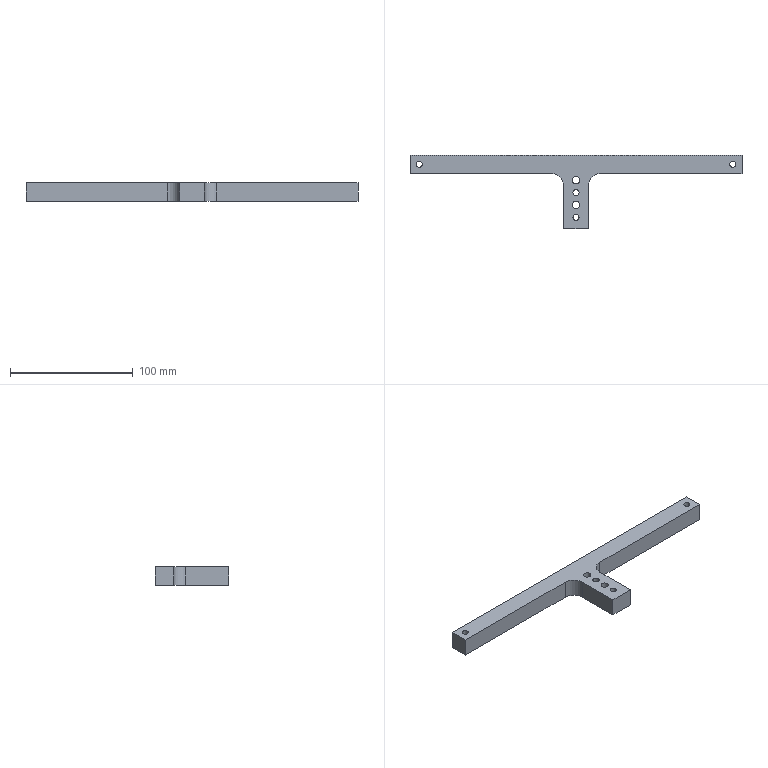Part | NX | features BREP 1 | 1 solid | 18 faces | box 270 x 60 x 15 mm | volume 72867 mm3 | plane 10 | cylinder 8 | commonest cylinder face diameters 5 x4 6 x2 20 x2
STEP:
#1=CARTESIAN_POINT('',(-10.,35.,7.5));
#2=VERTEX_POINT('',#1);
#3=CARTESIAN_POINT('',(-10.,0.,7.5));
#4=VERTEX_POINT('',#3);
#5=CARTESIAN_POINT('',(-10.,45.,7.5));
#6=DIRECTION('',(0.,-1.,0.));
#7=VECTOR('',#6,1000.);
#8=LINE('',#5,#7);
#9=EDGE_CURVE('',#2,#4,#8,.T.);
#10=ORIENTED_EDGE('',*,*,#9,.F.);
#11=CARTESIAN_POINT('',(-10.,35.,-7.5));
#12=VERTEX_POINT('',#11);
#13=CARTESIAN_POINT('',(-10.,35.,-7.5));
#14=DIRECTION('',(0.,0.,-1.));
#15=VECTOR('',#14,1000.);
#16=LINE('',#13,#15);
#17=EDGE_CURVE('',#2,#12,#16,.T.);
#18=ORIENTED_EDGE('',*,*,#17,.T.);
#19=CARTESIAN_POINT('',(-10.,0.,-7.5));
#20=VERTEX_POINT('',#19);
#21=CARTESIAN_POINT('',(-10.,45.,-7.5));
#22=DIRECTION('',(0.,-1.,0.));
#23=VECTOR('',#22,1000.);
#24=LINE('',#21,#23);
#25=EDGE_CURVE('',#12,#20,#24,.T.);
#26=ORIENTED_EDGE('',*,*,#25,.T.);
#27=CARTESIAN_POINT('',(-10.,0.,7.5));
#28=DIRECTION('',(0.,0.,-1.));
#29=VECTOR('',#28,1000.);
#30=LINE('',#27,#29);
#31=EDGE_CURVE('',#4,#20,#30,.T.);
#32=ORIENTED_EDGE('',*,*,#31,.F.);
#33=EDGE_LOOP('',(#10,#18,#26,#32));
#34=FACE_BOUND('',#33,.T.);
#35=CARTESIAN_POINT('',(-10.,45.,7.5));
#36=DIRECTION('',(1.,0.,0.));
#37=DIRECTION('',(0.,-1.,0.));
#38=AXIS2_PLACEMENT_3D('',#35,#36,#37);
#39=PLANE('',#38);
#40=ADVANCED_FACE('',(#34),#39,.F.);
#41=CARTESIAN_POINT('',(10.,0.,-7.5));
#42=VERTEX_POINT('',#41);
#43=CARTESIAN_POINT('',(-10.,0.,-7.5));
#44=DIRECTION('',(1.,0.,0.));
#45=VECTOR('',#44,1000.);
#46=LINE('',#43,#45);
#47=EDGE_CURVE('',#20,#42,#46,.T.);
#48=ORIENTED_EDGE('',*,*,#47,.T.);
#49=CARTESIAN_POINT('',(10.,0.,7.5));
#50=VERTEX_POINT('',#49);
#51=CARTESIAN_POINT('',(10.,0.,7.5));
#52=DIRECTION('',(0.,0.,-1.));
#53=VECTOR('',#52,1000.);
#54=LINE('',#51,#53);
#55=EDGE_CURVE('',#50,#42,#54,.T.);
#56=ORIENTED_EDGE('',*,*,#55,.F.);
#57=CARTESIAN_POINT('',(-10.,0.,7.5));
#58=DIRECTION('',(1.,0.,0.));
#59=VECTOR('',#58,1000.);
#60=LINE('',#57,#59);
#61=EDGE_CURVE('',#4,#50,#60,.T.);
#62=ORIENTED_EDGE('',*,*,#61,.F.);
#63=ORIENTED_EDGE('',*,*,#31,.T.);
#64=EDGE_LOOP('',(#48,#56,#62,#63));
#65=FACE_BOUND('',#64,.T.);
#66=CARTESIAN_POINT('',(-10.,0.,7.5));
#67=DIRECTION('',(0.,1.,0.));
#68=DIRECTION('',(0.,0.,-1.));
#69=AXIS2_PLACEMENT_3D('',#66,#67,#68);
#70=PLANE('',#69);
#71=ADVANCED_FACE('',(#65),#70,.F.);
#72=CARTESIAN_POINT('',(10.,35.,-7.5));
#73=VERTEX_POINT('',#72);
#74=CARTESIAN_POINT('',(10.,0.,-7.5));
#75=DIRECTION('',(0.,1.,0.));
#76=VECTOR('',#75,1000.);
#77=LINE('',#74,#76);
#78=EDGE_CURVE('',#42,#73,#77,.T.);
#79=ORIENTED_EDGE('',*,*,#78,.T.);
#80=CARTESIAN_POINT('',(10.,35.,7.5));
#81=VERTEX_POINT('',#80);
#82=CARTESIAN_POINT('',(10.,35.,7.5));
#83=DIRECTION('',(0.,0.,1.));
#84=VECTOR('',#83,1000.);
#85=LINE('',#82,#84);
#86=EDGE_CURVE('',#73,#81,#85,.T.);
#87=ORIENTED_EDGE('',*,*,#86,.T.);
#88=CARTESIAN_POINT('',(10.,0.,7.5));
#89=DIRECTION('',(0.,1.,0.));
#90=VECTOR('',#89,1000.);
#91=LINE('',#88,#90);
#92=EDGE_CURVE('',#50,#81,#91,.T.);
#93=ORIENTED_EDGE('',*,*,#92,.F.);
#94=ORIENTED_EDGE('',*,*,#55,.T.);
#95=EDGE_LOOP('',(#79,#87,#93,#94));
#96=FACE_BOUND('',#95,.T.);
#97=CARTESIAN_POINT('',(10.,0.,7.5));
#98=DIRECTION('',(-1.,0.,0.));
#99=DIRECTION('',(0.,1.,0.));
#100=AXIS2_PLACEMENT_3D('',#97,#98,#99);
#101=PLANE('',#100);
#102=ADVANCED_FACE('',(#96),#101,.F.);
#103=CARTESIAN_POINT('',(20.,45.,7.5));
#104=VERTEX_POINT('',#103);
#105=CARTESIAN_POINT('',(135.,45.,7.5));
#106=VERTEX_POINT('',#105);
#107=CARTESIAN_POINT('',(10.,45.,7.5));
#108=DIRECTION('',(1.,0.,0.));
#109=VECTOR('',#108,1000.);
#110=LINE('',#107,#109);
#111=EDGE_CURVE('',#104,#106,#110,.T.);
#112=ORIENTED_EDGE('',*,*,#111,.F.);
#113=CARTESIAN_POINT('',(20.,45.,-7.5));
#114=VERTEX_POINT('',#113);
#115=CARTESIAN_POINT('',(20.,45.,-7.5));
#116=DIRECTION('',(0.,0.,-1.));
#117=VECTOR('',#116,1000.);
#118=LINE('',#115,#117);
#119=EDGE_CURVE('',#104,#114,#118,.T.);
#120=ORIENTED_EDGE('',*,*,#119,.T.);
#121=CARTESIAN_POINT('',(135.,45.,-7.5));
#122=VERTEX_POINT('',#121);
#123=CARTESIAN_POINT('',(10.,45.,-7.5));
#124=DIRECTION('',(1.,0.,0.));
#125=VECTOR('',#124,1000.);
#126=LINE('',#123,#125);
#127=EDGE_CURVE('',#114,#122,#126,.T.);
#128=ORIENTED_EDGE('',*,*,#127,.T.);
#129=CARTESIAN_POINT('',(135.,45.,7.5));
#130=DIRECTION('',(0.,0.,-1.));
#131=VECTOR('',#130,1000.);
#132=LINE('',#129,#131);
#133=EDGE_CURVE('',#106,#122,#132,.T.);
#134=ORIENTED_EDGE('',*,*,#133,.F.);
#135=EDGE_LOOP('',(#112,#120,#128,#134));
#136=FACE_BOUND('',#135,.T.);
#137=CARTESIAN_POINT('',(10.,45.,7.5));
#138=DIRECTION('',(0.,1.,0.));
#139=DIRECTION('',(0.,0.,-1.));
#140=AXIS2_PLACEMENT_3D('',#137,#138,#139);
#141=PLANE('',#140);
#142=ADVANCED_FACE('',(#136),#141,.F.);
#143=CARTESIAN_POINT('',(135.,60.,-7.5));
#144=VERTEX_POINT('',#143);
#145=CARTESIAN_POINT('',(135.,45.,-7.5));
#146=DIRECTION('',(0.,1.,0.));
#147=VECTOR('',#146,1000.);
#148=LINE('',#145,#147);
#149=EDGE_CURVE('',#122,#144,#148,.T.);
#150=ORIENTED_EDGE('',*,*,#149,.T.);
#151=CARTESIAN_POINT('',(135.,60.,7.5));
#152=VERTEX_POINT('',#151);
#153=CARTESIAN_POINT('',(135.,60.,7.5));
#154=DIRECTION('',(0.,0.,-1.));
#155=VECTOR('',#154,1000.);
#156=LINE('',#153,#155);
#157=EDGE_CURVE('',#152,#144,#156,.T.);
#158=ORIENTED_EDGE('',*,*,#157,.F.);
#159=CARTESIAN_POINT('',(135.,45.,7.5));
#160=DIRECTION('',(0.,1.,0.));
#161=VECTOR('',#160,1000.);
#162=LINE('',#159,#161);
#163=EDGE_CURVE('',#106,#152,#162,.T.);
#164=ORIENTED_EDGE('',*,*,#163,.F.);
#165=ORIENTED_EDGE('',*,*,#133,.T.);
#166=EDGE_LOOP('',(#150,#158,#164,#165));
#167=FACE_BOUND('',#166,.T.);
#168=CARTESIAN_POINT('',(135.,45.,7.5));
#169=DIRECTION('',(-1.,0.,0.));
#170=DIRECTION('',(0.,0.,-1.));
#171=AXIS2_PLACEMENT_3D('',#168,#169,#170);
#172=PLANE('',#171);
#173=ADVANCED_FACE('',(#167),#172,.F.);
#174=CARTESIAN_POINT('',(-135.,60.,-7.5));
#175=VERTEX_POINT('',#174);
#176=CARTESIAN_POINT('',(135.,60.,-7.5));
#177=DIRECTION('',(-1.,0.,0.));
#178=VECTOR('',#177,1000.);
#179=LINE('',#176,#178);
#180=EDGE_CURVE('',#144,#175,#179,.T.);
#181=ORIENTED_EDGE('',*,*,#180,.T.);
#182=CARTESIAN_POINT('',(-135.,60.,7.5));
#183=VERTEX_POINT('',#182);
#184=CARTESIAN_POINT('',(-135.,60.,7.5));
#185=DIRECTION('',(0.,0.,-1.));
#186=VECTOR('',#185,1000.);
#187=LINE('',#184,#186);
#188=EDGE_CURVE('',#183,#175,#187,.T.);
#189=ORIENTED_EDGE('',*,*,#188,.F.);
#190=CARTESIAN_POINT('',(135.,60.,7.5));
#191=DIRECTION('',(-1.,0.,0.));
#192=VECTOR('',#191,1000.);
#193=LINE('',#190,#192);
#194=EDGE_CURVE('',#152,#183,#193,.T.);
#195=ORIENTED_EDGE('',*,*,#194,.F.);
#196=ORIENTED_EDGE('',*,*,#157,.T.);
#197=EDGE_LOOP('',(#181,#189,#195,#196));
#198=FACE_BOUND('',#197,.T.);
#199=CARTESIAN_POINT('',(135.,60.,7.5));
#200=DIRECTION('',(0.,-1.,0.));
#201=DIRECTION('',(0.,0.,1.));
#202=AXIS2_PLACEMENT_3D('',#199,#200,#201);
#203=PLANE('',#202);
#204=ADVANCED_FACE('',(#198),#203,.F.);
#205=CARTESIAN_POINT('',(-135.,45.,-7.5));
#206=VERTEX_POINT('',#205);
#207=CARTESIAN_POINT('',(-135.,60.,-7.5));
#208=DIRECTION('',(0.,-1.,0.));
#209=VECTOR('',#208,1000.);
#210=LINE('',#207,#209);
#211=EDGE_CURVE('',#175,#206,#210,.T.);
#212=ORIENTED_EDGE('',*,*,#211,.T.);
#213=CARTESIAN_POINT('',(-135.,45.,7.5));
#214=VERTEX_POINT('',#213);
#215=CARTESIAN_POINT('',(-135.,45.,7.5));
#216=DIRECTION('',(0.,0.,-1.));
#217=VECTOR('',#216,1000.);
#218=LINE('',#215,#217);
#219=EDGE_CURVE('',#214,#206,#218,.T.);
#220=ORIENTED_EDGE('',*,*,#219,.F.);
#221=CARTESIAN_POINT('',(-135.,60.,7.5));
#222=DIRECTION('',(0.,-1.,0.));
#223=VECTOR('',#222,1000.);
#224=LINE('',#221,#223);
#225=EDGE_CURVE('',#183,#214,#224,.T.);
#226=ORIENTED_EDGE('',*,*,#225,.F.);
#227=ORIENTED_EDGE('',*,*,#188,.T.);
#228=EDGE_LOOP('',(#212,#220,#226,#227));
#229=FACE_BOUND('',#228,.T.);
#230=CARTESIAN_POINT('',(-135.,60.,7.5));
#231=DIRECTION('',(1.,0.,0.));
#232=DIRECTION('',(0.,0.,1.));
#233=AXIS2_PLACEMENT_3D('',#230,#231,#232);
#234=PLANE('',#233);
#235=ADVANCED_FACE('',(#229),#234,.F.);
#236=CARTESIAN_POINT('',(-20.,45.,-7.5));
#237=VERTEX_POINT('',#236);
#238=CARTESIAN_POINT('',(-135.,45.,-7.5));
#239=DIRECTION('',(1.,0.,0.));
#240=VECTOR('',#239,1000.);
#241=LINE('',#238,#240);
#242=EDGE_CURVE('',#206,#237,#241,.T.);
#243=ORIENTED_EDGE('',*,*,#242,.T.);
#244=CARTESIAN_POINT('',(-20.,45.,7.5));
#245=VERTEX_POINT('',#244);
#246=CARTESIAN_POINT('',(-20.,45.,7.5));
#247=DIRECTION('',(0.,0.,1.));
#248=VECTOR('',#247,1000.);
#249=LINE('',#246,#248);
#250=EDGE_CURVE('',#237,#245,#249,.T.);
#251=ORIENTED_EDGE('',*,*,#250,.T.);
#252=CARTESIAN_POINT('',(-135.,45.,7.5));
#253=DIRECTION('',(1.,0.,0.));
#254=VECTOR('',#253,1000.);
#255=LINE('',#252,#254);
#256=EDGE_CURVE('',#214,#245,#255,.T.);
#257=ORIENTED_EDGE('',*,*,#256,.F.);
#258=ORIENTED_EDGE('',*,*,#219,.T.);
#259=EDGE_LOOP('',(#243,#251,#257,#258));
#260=FACE_BOUND('',#259,.T.);
#261=CARTESIAN_POINT('',(-135.,45.,7.5));
#262=DIRECTION('',(0.,1.,0.));
#263=DIRECTION('',(0.,0.,-1.));
#264=AXIS2_PLACEMENT_3D('',#261,#262,#263);
#265=PLANE('',#264);
#266=ADVANCED_FACE('',(#260),#265,.F.);
#267=CARTESIAN_POINT('',(-125.,52.5,7.5));
#268=VERTEX_POINT('',#267);
#269=CARTESIAN_POINT('',(-127.5,52.5,7.5));
#270=DIRECTION('',(0.,0.,1.));
#271=DIRECTION('',(1.,0.,0.));
#272=AXIS2_PLACEMENT_3D('',#269,#270,#271);
#273=CIRCLE('',#272,2.5);
#274=EDGE_CURVE('',#268,#268,#273,.T.);
#275=ORIENTED_EDGE('',*,*,#274,.F.);
#276=EDGE_LOOP('',(#275));
#277=FACE_BOUND('',#276,.T.);
#278=CARTESIAN_POINT('',(130.,52.5,7.5));
#279=VERTEX_POINT('',#278);
#280=CARTESIAN_POINT('',(127.5,52.5,7.5));
#281=DIRECTION('',(0.,0.,1.));
#282=DIRECTION('',(1.,0.,0.));
#283=AXIS2_PLACEMENT_3D('',#280,#281,#282);
#284=CIRCLE('',#283,2.5);
#285=EDGE_CURVE('',#279,#279,#284,.T.);
#286=ORIENTED_EDGE('',*,*,#285,.F.);
#287=EDGE_LOOP('',(#286));
#288=FACE_BOUND('',#287,.T.);
#289=CARTESIAN_POINT('',(-2.5,9.5,7.5));
#290=VERTEX_POINT('',#289);
#291=CARTESIAN_POINT('',(0.,9.5,7.5));
#292=DIRECTION('',(0.,0.,-1.));
#293=DIRECTION('',(-1.,0.,0.));
#294=AXIS2_PLACEMENT_3D('',#291,#292,#293);
#295=CIRCLE('',#294,2.5);
#296=EDGE_CURVE('',#290,#290,#295,.T.);
#297=ORIENTED_EDGE('',*,*,#296,.T.);
#298=EDGE_LOOP('',(#297));
#299=FACE_BOUND('',#298,.T.);
#300=CARTESIAN_POINT('',(-2.5,29.5,7.5));
#301=VERTEX_POINT('',#300);
#302=CARTESIAN_POINT('',(0.,29.5,7.5));
#303=DIRECTION('',(0.,0.,-1.));
#304=DIRECTION('',(-1.,0.,0.));
#305=AXIS2_PLACEMENT_3D('',#302,#303,#304);
#306=CIRCLE('',#305,2.5);
#307=EDGE_CURVE('',#301,#301,#306,.T.);
#308=ORIENTED_EDGE('',*,*,#307,.T.);
#309=EDGE_LOOP('',(#308));
#310=FACE_BOUND('',#309,.T.);
#311=CARTESIAN_POINT('',(3.,19.5,7.5));
#312=VERTEX_POINT('',#311);
#313=CARTESIAN_POINT('',(0.,19.5,7.5));
#314=DIRECTION('',(0.,0.,1.));
#315=DIRECTION('',(1.,0.,0.));
#316=AXIS2_PLACEMENT_3D('',#313,#314,#315);
#317=CIRCLE('',#316,3.);
#318=EDGE_CURVE('',#312,#312,#317,.T.);
#319=ORIENTED_EDGE('',*,*,#318,.F.);
#320=EDGE_LOOP('',(#319));
#321=FACE_BOUND('',#320,.T.);
#322=CARTESIAN_POINT('',(3.,39.5,7.5));
#323=VERTEX_POINT('',#322);
#324=CARTESIAN_POINT('',(0.,39.5,7.5));
#325=DIRECTION('',(0.,0.,1.));
#326=DIRECTION('',(1.,0.,0.));
#327=AXIS2_PLACEMENT_3D('',#324,#325,#326);
#328=CIRCLE('',#327,3.);
#329=EDGE_CURVE('',#323,#323,#328,.T.);
#330=ORIENTED_EDGE('',*,*,#329,.F.);
#331=EDGE_LOOP('',(#330));
#332=FACE_BOUND('',#331,.T.);
#333=ORIENTED_EDGE('',*,*,#256,.T.);
#334=CARTESIAN_POINT('',(-20.,35.,7.5));
#335=DIRECTION('',(0.,0.,-1.));
#336=DIRECTION('',(1.,0.,0.));
#337=AXIS2_PLACEMENT_3D('',#334,#335,#336);
#338=CIRCLE('',#337,10.);
#339=EDGE_CURVE('',#245,#2,#338,.T.);
#340=ORIENTED_EDGE('',*,*,#339,.T.);
#341=ORIENTED_EDGE('',*,*,#9,.T.);
#342=ORIENTED_EDGE('',*,*,#61,.T.);
#343=ORIENTED_EDGE('',*,*,#92,.T.);
#344=CARTESIAN_POINT('',(20.,35.,7.5));
#345=DIRECTION('',(0.,0.,-1.));
#346=DIRECTION('',(1.,0.,0.));
#347=AXIS2_PLACEMENT_3D('',#344,#345,#346);
#348=CIRCLE('',#347,10.);
#349=EDGE_CURVE('',#81,#104,#348,.T.);
#350=ORIENTED_EDGE('',*,*,#349,.T.);
#351=ORIENTED_EDGE('',*,*,#111,.T.);
#352=ORIENTED_EDGE('',*,*,#163,.T.);
#353=ORIENTED_EDGE('',*,*,#194,.T.);
#354=ORIENTED_EDGE('',*,*,#225,.T.);
#355=EDGE_LOOP('',(#333,#340,#341,#342,#343,#350,#351,#352,#353,#354));
#356=FACE_BOUND('',#355,.T.);
#357=CARTESIAN_POINT('',(0.,0.,7.5));
#358=DIRECTION('',(0.,0.,1.));
#359=DIRECTION('',(-1.,0.,0.));
#360=AXIS2_PLACEMENT_3D('',#357,#358,#359);
#361=PLANE('',#360);
#362=ADVANCED_FACE('',(#277,#288,#299,#310,#321,#332,#356),#361,.T.);
#363=CARTESIAN_POINT('',(-125.,52.5,-7.5));
#364=VERTEX_POINT('',#363);
#365=CARTESIAN_POINT('',(-127.5,52.5,-7.5));
#366=DIRECTION('',(0.,0.,1.));
#367=DIRECTION('',(1.,0.,0.));
#368=AXIS2_PLACEMENT_3D('',#365,#366,#367);
#369=CIRCLE('',#368,2.5);
#370=EDGE_CURVE('',#364,#364,#369,.T.);
#371=ORIENTED_EDGE('',*,*,#370,.T.);
#372=EDGE_LOOP('',(#371));
#373=FACE_BOUND('',#372,.T.);
#374=CARTESIAN_POINT('',(130.,52.5,-7.5));
#375=VERTEX_POINT('',#374);
#376=CARTESIAN_POINT('',(127.5,52.5,-7.5));
#377=DIRECTION('',(0.,0.,1.));
#378=DIRECTION('',(1.,0.,0.));
#379=AXIS2_PLACEMENT_3D('',#376,#377,#378);
#380=CIRCLE('',#379,2.5);
#381=EDGE_CURVE('',#375,#375,#380,.T.);
#382=ORIENTED_EDGE('',*,*,#381,.T.);
#383=EDGE_LOOP('',(#382));
#384=FACE_BOUND('',#383,.T.);
#385=CARTESIAN_POINT('',(-2.5,9.5,-7.5));
#386=VERTEX_POINT('',#385);
#387=CARTESIAN_POINT('',(0.,9.5,-7.5));
#388=DIRECTION('',(0.,0.,-1.));
#389=DIRECTION('',(-1.,0.,0.));
#390=AXIS2_PLACEMENT_3D('',#387,#388,#389);
#391=CIRCLE('',#390,2.5);
#392=EDGE_CURVE('',#386,#386,#391,.T.);
#393=ORIENTED_EDGE('',*,*,#392,.F.);
#394=EDGE_LOOP('',(#393));
#395=FACE_BOUND('',#394,.T.);
#396=CARTESIAN_POINT('',(-2.5,29.5,-7.5));
#397=VERTEX_POINT('',#396);
#398=CARTESIAN_POINT('',(0.,29.5,-7.5));
#399=DIRECTION('',(0.,0.,-1.));
#400=DIRECTION('',(-1.,0.,0.));
#401=AXIS2_PLACEMENT_3D('',#398,#399,#400);
#402=CIRCLE('',#401,2.5);
#403=EDGE_CURVE('',#397,#397,#402,.T.);
#404=ORIENTED_EDGE('',*,*,#403,.F.);
#405=EDGE_LOOP('',(#404));
#406=FACE_BOUND('',#405,.T.);
#407=CARTESIAN_POINT('',(-3.,19.5,-7.5));
#408=VERTEX_POINT('',#407);
#409=CARTESIAN_POINT('',(0.,19.5,-7.5));
#410=DIRECTION('',(0.,0.,-1.));
#411=DIRECTION('',(-1.,0.,0.));
#412=AXIS2_PLACEMENT_3D('',#409,#410,#411);
#413=CIRCLE('',#412,3.);
#414=EDGE_CURVE('',#408,#408,#413,.T.);
#415=ORIENTED_EDGE('',*,*,#414,.F.);
#416=EDGE_LOOP('',(#415));
#417=FACE_BOUND('',#416,.T.);
#418=CARTESIAN_POINT('',(-3.,39.5,-7.5));
#419=VERTEX_POINT('',#418);
#420=CARTESIAN_POINT('',(0.,39.5,-7.5));
#421=DIRECTION('',(0.,0.,-1.));
#422=DIRECTION('',(-1.,0.,0.));
#423=AXIS2_PLACEMENT_3D('',#420,#421,#422);
#424=CIRCLE('',#423,3.);
#425=EDGE_CURVE('',#419,#419,#424,.T.);
#426=ORIENTED_EDGE('',*,*,#425,.F.);
#427=EDGE_LOOP('',(#426));
#428=FACE_BOUND('',#427,.T.);
#429=ORIENTED_EDGE('',*,*,#25,.F.);
#430=CARTESIAN_POINT('',(-20.,35.,-7.5));
#431=DIRECTION('',(0.,0.,1.));
#432=DIRECTION('',(1.,0.,0.));
#433=AXIS2_PLACEMENT_3D('',#430,#431,#432);
#434=CIRCLE('',#433,10.);
#435=EDGE_CURVE('',#12,#237,#434,.T.);
#436=ORIENTED_EDGE('',*,*,#435,.T.);
#437=ORIENTED_EDGE('',*,*,#242,.F.);
#438=ORIENTED_EDGE('',*,*,#211,.F.);
#439=ORIENTED_EDGE('',*,*,#180,.F.);
#440=ORIENTED_EDGE('',*,*,#149,.F.);
#441=ORIENTED_EDGE('',*,*,#127,.F.);
#442=CARTESIAN_POINT('',(20.,35.,-7.5));
#443=DIRECTION('',(0.,0.,1.));
#444=DIRECTION('',(1.,0.,0.));
#445=AXIS2_PLACEMENT_3D('',#442,#443,#444);
#446=CIRCLE('',#445,10.);
#447=EDGE_CURVE('',#114,#73,#446,.T.);
#448=ORIENTED_EDGE('',*,*,#447,.T.);
#449=ORIENTED_EDGE('',*,*,#78,.F.);
#450=ORIENTED_EDGE('',*,*,#47,.F.);
#451=EDGE_LOOP('',(#429,#436,#437,#438,#439,#440,#441,#448,#449,#450));
#452=FACE_BOUND('',#451,.T.);
#453=CARTESIAN_POINT('',(0.,0.,-7.5));
#454=DIRECTION('',(0.,0.,1.));
#455=DIRECTION('',(-1.,0.,0.));
#456=AXIS2_PLACEMENT_3D('',#453,#454,#455);
#457=PLANE('',#456);
#458=ADVANCED_FACE('',(#373,#384,#395,#406,#417,#428,#452),#457,.F.);
#459=ORIENTED_EDGE('',*,*,#329,.T.);
#460=EDGE_LOOP('',(#459));
#461=FACE_BOUND('',#460,.T.);
#462=ORIENTED_EDGE('',*,*,#425,.T.);
#463=EDGE_LOOP('',(#462));
#464=FACE_BOUND('',#463,.T.);
#465=CARTESIAN_POINT('',(0.,39.5,-7.5));
#466=DIRECTION('',(0.,0.,-1.));
#467=DIRECTION('',(1.,0.,0.));
#468=AXIS2_PLACEMENT_3D('',#465,#466,#467);
#469=CYLINDRICAL_SURFACE('',#468,3.);
#470=ADVANCED_FACE('',(#461,#464),#469,.F.);
#471=ORIENTED_EDGE('',*,*,#318,.T.);
#472=EDGE_LOOP('',(#471));
#473=FACE_BOUND('',#472,.T.);
#474=ORIENTED_EDGE('',*,*,#414,.T.);
#475=EDGE_LOOP('',(#474));
#476=FACE_BOUND('',#475,.T.);
#477=CARTESIAN_POINT('',(0.,19.5,-7.5));
#478=DIRECTION('',(0.,0.,-1.));
#479=DIRECTION('',(1.,0.,0.));
#480=AXIS2_PLACEMENT_3D('',#477,#478,#479);
#481=CYLINDRICAL_SURFACE('',#480,3.);
#482=ADVANCED_FACE('',(#473,#476),#481,.F.);
#483=ORIENTED_EDGE('',*,*,#307,.F.);
#484=EDGE_LOOP('',(#483));
#485=FACE_BOUND('',#484,.T.);
#486=ORIENTED_EDGE('',*,*,#403,.T.);
#487=EDGE_LOOP('',(#486));
#488=FACE_BOUND('',#487,.T.);
#489=CARTESIAN_POINT('',(0.,29.5,-7.5));
#490=DIRECTION('',(0.,0.,-1.));
#491=DIRECTION('',(1.,0.,0.));
#492=AXIS2_PLACEMENT_3D('',#489,#490,#491);
#493=CYLINDRICAL_SURFACE('',#492,2.5);
#494=ADVANCED_FACE('',(#485,#488),#493,.F.);
#495=ORIENTED_EDGE('',*,*,#296,.F.);
#496=EDGE_LOOP('',(#495));
#497=FACE_BOUND('',#496,.T.);
#498=ORIENTED_EDGE('',*,*,#392,.T.);
#499=EDGE_LOOP('',(#498));
#500=FACE_BOUND('',#499,.T.);
#501=CARTESIAN_POINT('',(0.,9.5,-7.5));
#502=DIRECTION('',(0.,0.,-1.));
#503=DIRECTION('',(1.,0.,0.));
#504=AXIS2_PLACEMENT_3D('',#501,#502,#503);
#505=CYLINDRICAL_SURFACE('',#504,2.5);
#506=ADVANCED_FACE('',(#497,#500),#505,.F.);
#507=ORIENTED_EDGE('',*,*,#381,.F.);
#508=EDGE_LOOP('',(#507));
#509=FACE_BOUND('',#508,.T.);
#510=ORIENTED_EDGE('',*,*,#285,.T.);
#511=EDGE_LOOP('',(#510));
#512=FACE_BOUND('',#511,.T.);
#513=CARTESIAN_POINT('',(127.5,52.5,7.5));
#514=DIRECTION('',(0.,0.,1.));
#515=DIRECTION('',(-1.,0.,0.));
#516=AXIS2_PLACEMENT_3D('',#513,#514,#515);
#517=CYLINDRICAL_SURFACE('',#516,2.5);
#518=ADVANCED_FACE('',(#509,#512),#517,.F.);
#519=ORIENTED_EDGE('',*,*,#370,.F.);
#520=EDGE_LOOP('',(#519));
#521=FACE_BOUND('',#520,.T.);
#522=ORIENTED_EDGE('',*,*,#274,.T.);
#523=EDGE_LOOP('',(#522));
#524=FACE_BOUND('',#523,.T.);
#525=CARTESIAN_POINT('',(-127.5,52.5,7.5));
#526=DIRECTION('',(0.,0.,1.));
#527=DIRECTION('',(-1.,0.,0.));
#528=AXIS2_PLACEMENT_3D('',#525,#526,#527);
#529=CYLINDRICAL_SURFACE('',#528,2.5);
#530=ADVANCED_FACE('',(#521,#524),#529,.F.);
#531=ORIENTED_EDGE('',*,*,#349,.F.);
#532=ORIENTED_EDGE('',*,*,#86,.F.);
#533=ORIENTED_EDGE('',*,*,#447,.F.);
#534=ORIENTED_EDGE('',*,*,#119,.F.);
#535=EDGE_LOOP('',(#531,#532,#533,#534));
#536=FACE_BOUND('',#535,.T.);
#537=CARTESIAN_POINT('',(20.,35.,7.5));
#538=DIRECTION('',(0.,0.,1.));
#539=DIRECTION('',(-1.,0.,0.));
#540=AXIS2_PLACEMENT_3D('',#537,#538,#539);
#541=CYLINDRICAL_SURFACE('',#540,10.);
#542=ADVANCED_FACE('',(#536),#541,.F.);
#543=ORIENTED_EDGE('',*,*,#339,.F.);
#544=ORIENTED_EDGE('',*,*,#250,.F.);
#545=ORIENTED_EDGE('',*,*,#435,.F.);
#546=ORIENTED_EDGE('',*,*,#17,.F.);
#547=EDGE_LOOP('',(#543,#544,#545,#546));
#548=FACE_BOUND('',#547,.T.);
#549=CARTESIAN_POINT('',(-20.,35.,7.5));
#550=DIRECTION('',(0.,0.,1.));
#551=DIRECTION('',(-1.,0.,0.));
#552=AXIS2_PLACEMENT_3D('',#549,#550,#551);
#553=CYLINDRICAL_SURFACE('',#552,10.);
#554=ADVANCED_FACE('',(#548),#553,.F.);
#555=CLOSED_SHELL('',(#40,#71,#102,#142,#173,#204,#235,#266,#362,#458,#470,#482,#494,#506,#518,#530,#542,#554));
#556=MANIFOLD_SOLID_BREP('',#555);
#557=(LENGTH_UNIT()NAMED_UNIT(*)SI_UNIT(.MILLI.,.METRE.));
#558=UNCERTAINTY_MEASURE_WITH_UNIT(LENGTH_MEASURE(0.00001),#557,'','');
#559=(NAMED_UNIT(*)PLANE_ANGLE_UNIT()SI_UNIT($,.RADIAN.));
#560=(NAMED_UNIT(*)SI_UNIT($,.STERADIAN.)SOLID_ANGLE_UNIT());
#561=(GEOMETRIC_REPRESENTATION_CONTEXT(3)GLOBAL_UNCERTAINTY_ASSIGNED_CONTEXT((#558))GLOBAL_UNIT_ASSIGNED_CONTEXT((#557,#559,#560))REPRESENTATION_CONTEXT('',''));
#562=ADVANCED_BREP_SHAPE_REPRESENTATION('',(#556),#561);